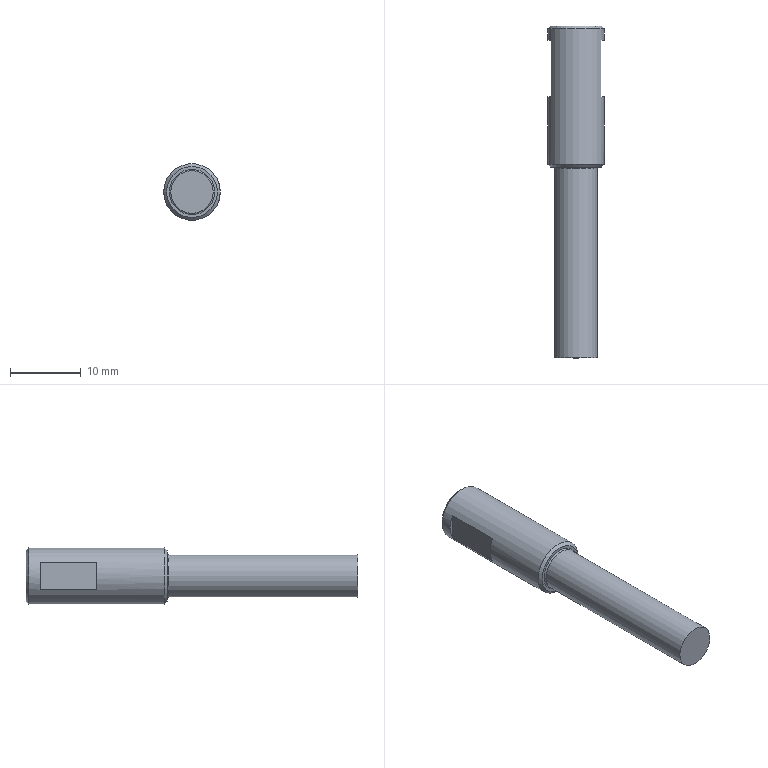Part | NX | features 5003_002_SFRNS8-20.0-F27.0-B13-P6-SC10 2 | 1 solid | 14 faces | box 8 x 47 x 8 mm | volume 1744 mm3 | plane 9 | cylinder 2 | cone 2 | torus 1 | commonest cylinder face diameters 6 x1 8 x1
STEP:
#1=CARTESIAN_POINT('',(-212.775,-579.,-110.5));
#2=VERTEX_POINT('',#1);
#3=CARTESIAN_POINT('',(-216.775,-579.,-110.5));
#4=DIRECTION('',(0.,-1.,0.));
#5=DIRECTION('',(1.,0.,0.));
#6=AXIS2_PLACEMENT_3D('',#3,#4,#5);
#7=CIRCLE('',#6,4.);
#8=EDGE_CURVE('',#2,#2,#7,.T.);
#9=ORIENTED_EDGE('',*,*,#8,.T.);
#10=EDGE_LOOP('',(#9));
#11=FACE_BOUND('',#10,.T.);
#12=CARTESIAN_POINT('',(-220.775,-598.2,-110.5));
#13=VERTEX_POINT('',#12);
#14=CARTESIAN_POINT('',(-216.775,-598.2,-110.5));
#15=DIRECTION('',(0.,1.,0.));
#16=DIRECTION('',(-1.,0.,0.));
#17=AXIS2_PLACEMENT_3D('',#14,#15,#16);
#18=CIRCLE('',#17,4.);
#19=EDGE_CURVE('',#13,#13,#18,.T.);
#20=ORIENTED_EDGE('',*,*,#19,.T.);
#21=EDGE_LOOP('',(#20));
#22=FACE_BOUND('',#21,.T.);
#23=CARTESIAN_POINT('',(-213.275,-580.6,-108.564));
#24=VERTEX_POINT('',#23);
#25=CARTESIAN_POINT('',(-213.275,-588.6,-108.564));
#26=VERTEX_POINT('',#25);
#27=CARTESIAN_POINT('',(-213.275,-625.6,-108.564));
#28=DIRECTION('',(0.,-1.,0.));
#29=VECTOR('',#28,1000.);
#30=LINE('',#27,#29);
#31=EDGE_CURVE('',#24,#26,#30,.T.);
#32=ORIENTED_EDGE('',*,*,#31,.F.);
#33=CARTESIAN_POINT('',(-213.275,-580.6,-112.436));
#34=VERTEX_POINT('',#33);
#35=CARTESIAN_POINT('',(-216.775,-580.6,-110.5));
#36=DIRECTION('',(0.,-1.,0.));
#37=DIRECTION('',(1.,0.,0.));
#38=AXIS2_PLACEMENT_3D('',#35,#36,#37);
#39=CIRCLE('',#38,4.);
#40=EDGE_CURVE('',#34,#24,#39,.T.);
#41=ORIENTED_EDGE('',*,*,#40,.F.);
#42=CARTESIAN_POINT('',(-213.275,-588.6,-112.436));
#43=VERTEX_POINT('',#42);
#44=CARTESIAN_POINT('',(-213.275,-625.6,-112.436));
#45=DIRECTION('',(0.,-1.,0.));
#46=VECTOR('',#45,1000.);
#47=LINE('',#44,#46);
#48=EDGE_CURVE('',#43,#34,#47,.F.);
#49=ORIENTED_EDGE('',*,*,#48,.F.);
#50=CARTESIAN_POINT('',(-216.775,-588.6,-110.5));
#51=DIRECTION('',(0.,1.,0.));
#52=DIRECTION('',(-1.,0.,0.));
#53=AXIS2_PLACEMENT_3D('',#50,#51,#52);
#54=CIRCLE('',#53,4.);
#55=EDGE_CURVE('',#26,#43,#54,.T.);
#56=ORIENTED_EDGE('',*,*,#55,.F.);
#57=EDGE_LOOP('',(#32,#41,#49,#56));
#58=FACE_BOUND('',#57,.T.);
#59=CARTESIAN_POINT('',(-220.275,-580.6,-108.564));
#60=VERTEX_POINT('',#59);
#61=CARTESIAN_POINT('',(-220.275,-580.6,-112.436));
#62=VERTEX_POINT('',#61);
#63=CARTESIAN_POINT('',(-216.775,-580.6,-110.5));
#64=DIRECTION('',(0.,-1.,0.));
#65=DIRECTION('',(1.,0.,0.));
#66=AXIS2_PLACEMENT_3D('',#63,#64,#65);
#67=CIRCLE('',#66,4.);
#68=EDGE_CURVE('',#60,#62,#67,.T.);
#69=ORIENTED_EDGE('',*,*,#68,.F.);
#70=CARTESIAN_POINT('',(-220.275,-588.6,-108.564));
#71=VERTEX_POINT('',#70);
#72=CARTESIAN_POINT('',(-220.275,-625.6,-108.564));
#73=DIRECTION('',(0.,-1.,0.));
#74=VECTOR('',#73,1000.);
#75=LINE('',#72,#74);
#76=EDGE_CURVE('',#71,#60,#75,.F.);
#77=ORIENTED_EDGE('',*,*,#76,.F.);
#78=CARTESIAN_POINT('',(-220.275,-588.6,-112.436));
#79=VERTEX_POINT('',#78);
#80=CARTESIAN_POINT('',(-216.775,-588.6,-110.5));
#81=DIRECTION('',(0.,1.,0.));
#82=DIRECTION('',(-1.,0.,0.));
#83=AXIS2_PLACEMENT_3D('',#80,#81,#82);
#84=CIRCLE('',#83,4.);
#85=EDGE_CURVE('',#79,#71,#84,.T.);
#86=ORIENTED_EDGE('',*,*,#85,.F.);
#87=CARTESIAN_POINT('',(-220.275,-625.6,-112.436));
#88=DIRECTION('',(0.,-1.,0.));
#89=VECTOR('',#88,1000.);
#90=LINE('',#87,#89);
#91=EDGE_CURVE('',#62,#79,#90,.T.);
#92=ORIENTED_EDGE('',*,*,#91,.F.);
#93=EDGE_LOOP('',(#69,#77,#86,#92));
#94=FACE_BOUND('',#93,.T.);
#95=CARTESIAN_POINT('',(-216.775,-625.6,-110.5));
#96=DIRECTION('',(0.,-1.,0.));
#97=DIRECTION('',(1.,0.,0.));
#98=AXIS2_PLACEMENT_3D('',#95,#96,#97);
#99=CYLINDRICAL_SURFACE('',#98,4.);
#100=ADVANCED_FACE('',(#11,#22,#58,#94),#99,.T.);
#101=CARTESIAN_POINT('',(-213.175,-578.6,-110.5));
#102=VERTEX_POINT('',#101);
#103=CARTESIAN_POINT('',(-216.775,-578.6,-110.5));
#104=DIRECTION('',(0.,-1.,0.));
#105=DIRECTION('',(1.,0.,0.));
#106=AXIS2_PLACEMENT_3D('',#103,#104,#105);
#107=CIRCLE('',#106,3.6);
#108=EDGE_CURVE('',#102,#102,#107,.F.);
#109=ORIENTED_EDGE('',*,*,#108,.T.);
#110=EDGE_LOOP('',(#109));
#111=FACE_BOUND('',#110,.T.);
#112=CARTESIAN_POINT('',(-216.775,-578.6,-110.5));
#113=DIRECTION('',(0.,-1.,0.));
#114=DIRECTION('',(1.,0.,0.));
#115=AXIS2_PLACEMENT_3D('',#112,#113,#114);
#116=PLANE('',#115);
#117=ADVANCED_FACE('',(#111),#116,.F.);
#118=CARTESIAN_POINT('',(-219.975,-598.6,-110.5));
#119=VERTEX_POINT('',#118);
#120=CARTESIAN_POINT('',(-216.775,-598.6,-110.5));
#121=DIRECTION('',(0.,1.,0.));
#122=DIRECTION('',(-1.,0.,0.));
#123=AXIS2_PLACEMENT_3D('',#120,#121,#122);
#124=CIRCLE('',#123,3.2);
#125=EDGE_CURVE('',#119,#119,#124,.T.);
#126=ORIENTED_EDGE('',*,*,#125,.T.);
#127=EDGE_LOOP('',(#126));
#128=FACE_BOUND('',#127,.T.);
#129=CARTESIAN_POINT('',(-220.375,-598.6,-110.5));
#130=VERTEX_POINT('',#129);
#131=CARTESIAN_POINT('',(-216.775,-598.6,-110.5));
#132=DIRECTION('',(0.,1.,0.));
#133=DIRECTION('',(-1.,0.,0.));
#134=AXIS2_PLACEMENT_3D('',#131,#132,#133);
#135=CIRCLE('',#134,3.6);
#136=EDGE_CURVE('',#130,#130,#135,.F.);
#137=ORIENTED_EDGE('',*,*,#136,.T.);
#138=EDGE_LOOP('',(#137));
#139=FACE_BOUND('',#138,.T.);
#140=CARTESIAN_POINT('',(-216.775,-598.6,-106.5));
#141=DIRECTION('',(0.,1.,0.));
#142=DIRECTION('',(-1.,0.,0.));
#143=AXIS2_PLACEMENT_3D('',#140,#141,#142);
#144=PLANE('',#143);
#145=ADVANCED_FACE('',(#128,#139),#144,.F.);
#146=CARTESIAN_POINT('',(-219.775,-598.8,-110.5));
#147=VERTEX_POINT('',#146);
#148=CARTESIAN_POINT('',(-216.775,-598.8,-110.5));
#149=DIRECTION('',(0.,1.,0.));
#150=DIRECTION('',(-1.,0.,0.));
#151=AXIS2_PLACEMENT_3D('',#148,#149,#150);
#152=CIRCLE('',#151,3.);
#153=EDGE_CURVE('',#147,#147,#152,.F.);
#154=ORIENTED_EDGE('',*,*,#153,.T.);
#155=EDGE_LOOP('',(#154));
#156=FACE_BOUND('',#155,.T.);
#157=CARTESIAN_POINT('',(-213.775,-625.6,-110.5));
#158=VERTEX_POINT('',#157);
#159=CARTESIAN_POINT('',(-216.775,-625.6,-110.5));
#160=DIRECTION('',(0.,-1.,0.));
#161=DIRECTION('',(1.,0.,0.));
#162=AXIS2_PLACEMENT_3D('',#159,#160,#161);
#163=CIRCLE('',#162,3.);
#164=EDGE_CURVE('',#158,#158,#163,.T.);
#165=ORIENTED_EDGE('',*,*,#164,.F.);
#166=EDGE_LOOP('',(#165));
#167=FACE_BOUND('',#166,.T.);
#168=CARTESIAN_POINT('',(-216.775,-625.6,-110.5));
#169=DIRECTION('',(0.,-1.,0.));
#170=DIRECTION('',(1.,0.,0.));
#171=AXIS2_PLACEMENT_3D('',#168,#169,#170);
#172=CYLINDRICAL_SURFACE('',#171,3.);
#173=ADVANCED_FACE('',(#156,#167),#172,.T.);
#174=ORIENTED_EDGE('',*,*,#164,.T.);
#175=EDGE_LOOP('',(#174));
#176=FACE_BOUND('',#175,.T.);
#177=CARTESIAN_POINT('',(-216.775,-625.6,-107.5));
#178=DIRECTION('',(0.,1.,0.));
#179=DIRECTION('',(-1.,0.,0.));
#180=AXIS2_PLACEMENT_3D('',#177,#178,#179);
#181=PLANE('',#180);
#182=ADVANCED_FACE('',(#176),#181,.F.);
#183=ORIENTED_EDGE('',*,*,#108,.F.);
#184=EDGE_LOOP('',(#183));
#185=FACE_BOUND('',#184,.T.);
#186=ORIENTED_EDGE('',*,*,#8,.F.);
#187=EDGE_LOOP('',(#186));
#188=FACE_BOUND('',#187,.T.);
#189=CARTESIAN_POINT('',(-216.775,-579.,-110.5));
#190=DIRECTION('',(0.,-1.,0.));
#191=DIRECTION('',(1.,0.,0.));
#192=AXIS2_PLACEMENT_3D('',#189,#190,#191);
#193=CONICAL_SURFACE('',#192,4.,0.7854);
#194=ADVANCED_FACE('',(#185,#188),#193,.T.);
#195=ORIENTED_EDGE('',*,*,#19,.F.);
#196=EDGE_LOOP('',(#195));
#197=FACE_BOUND('',#196,.T.);
#198=ORIENTED_EDGE('',*,*,#136,.F.);
#199=EDGE_LOOP('',(#198));
#200=FACE_BOUND('',#199,.T.);
#201=CARTESIAN_POINT('',(-216.775,-598.6,-110.5));
#202=DIRECTION('',(0.,1.,0.));
#203=DIRECTION('',(-1.,0.,0.));
#204=AXIS2_PLACEMENT_3D('',#201,#202,#203);
#205=CONICAL_SURFACE('',#204,3.6,0.7854);
#206=ADVANCED_FACE('',(#197,#200),#205,.T.);
#207=ORIENTED_EDGE('',*,*,#125,.F.);
#208=EDGE_LOOP('',(#207));
#209=FACE_BOUND('',#208,.T.);
#210=ORIENTED_EDGE('',*,*,#153,.F.);
#211=EDGE_LOOP('',(#210));
#212=FACE_BOUND('',#211,.T.);
#213=CARTESIAN_POINT('',(-216.775,-598.8,-110.5));
#214=DIRECTION('',(0.,1.,0.));
#215=DIRECTION('',(-1.,0.,0.));
#216=AXIS2_PLACEMENT_3D('',#213,#214,#215);
#217=TOROIDAL_SURFACE('',#216,3.2,0.2);
#218=ADVANCED_FACE('',(#209,#212),#217,.F.);
#219=CARTESIAN_POINT('',(-213.275,-588.6,-106.5));
#220=DIRECTION('',(0.,0.,-1.));
#221=VECTOR('',#220,1000.);
#222=LINE('',#219,#221);
#223=EDGE_CURVE('',#26,#43,#222,.T.);
#224=ORIENTED_EDGE('',*,*,#223,.F.);
#225=ORIENTED_EDGE('',*,*,#55,.T.);
#226=EDGE_LOOP('',(#224,#225));
#227=FACE_BOUND('',#226,.T.);
#228=CARTESIAN_POINT('',(-213.275,-588.6,-106.5));
#229=DIRECTION('',(0.,1.,0.));
#230=DIRECTION('',(-1.,0.,0.));
#231=AXIS2_PLACEMENT_3D('',#228,#229,#230);
#232=PLANE('',#231);
#233=ADVANCED_FACE('',(#227),#232,.T.);
#234=ORIENTED_EDGE('',*,*,#40,.T.);
#235=CARTESIAN_POINT('',(-213.275,-580.6,-106.5));
#236=DIRECTION('',(0.,0.,-1.));
#237=VECTOR('',#236,1000.);
#238=LINE('',#235,#237);
#239=EDGE_CURVE('',#24,#34,#238,.T.);
#240=ORIENTED_EDGE('',*,*,#239,.T.);
#241=EDGE_LOOP('',(#234,#240));
#242=FACE_BOUND('',#241,.T.);
#243=CARTESIAN_POINT('',(-213.275,-580.6,-106.5));
#244=DIRECTION('',(0.,-1.,0.));
#245=DIRECTION('',(1.,0.,0.));
#246=AXIS2_PLACEMENT_3D('',#243,#244,#245);
#247=PLANE('',#246);
#248=ADVANCED_FACE('',(#242),#247,.T.);
#249=ORIENTED_EDGE('',*,*,#31,.T.);
#250=ORIENTED_EDGE('',*,*,#223,.T.);
#251=ORIENTED_EDGE('',*,*,#48,.T.);
#252=ORIENTED_EDGE('',*,*,#239,.F.);
#253=EDGE_LOOP('',(#249,#250,#251,#252));
#254=FACE_BOUND('',#253,.T.);
#255=CARTESIAN_POINT('',(-213.275,-588.6,-106.5));
#256=DIRECTION('',(1.,0.,0.));
#257=DIRECTION('',(0.,1.,0.));
#258=AXIS2_PLACEMENT_3D('',#255,#256,#257);
#259=PLANE('',#258);
#260=ADVANCED_FACE('',(#254),#259,.T.);
#261=ORIENTED_EDGE('',*,*,#85,.T.);
#262=CARTESIAN_POINT('',(-220.275,-588.6,-106.5));
#263=DIRECTION('',(0.,0.,-1.));
#264=VECTOR('',#263,1000.);
#265=LINE('',#262,#264);
#266=EDGE_CURVE('',#71,#79,#265,.T.);
#267=ORIENTED_EDGE('',*,*,#266,.T.);
#268=EDGE_LOOP('',(#261,#267));
#269=FACE_BOUND('',#268,.T.);
#270=CARTESIAN_POINT('',(-220.775,-588.6,-106.5));
#271=DIRECTION('',(0.,1.,0.));
#272=DIRECTION('',(-1.,0.,0.));
#273=AXIS2_PLACEMENT_3D('',#270,#271,#272);
#274=PLANE('',#273);
#275=ADVANCED_FACE('',(#269),#274,.T.);
#276=ORIENTED_EDGE('',*,*,#91,.T.);
#277=ORIENTED_EDGE('',*,*,#266,.F.);
#278=ORIENTED_EDGE('',*,*,#76,.T.);
#279=CARTESIAN_POINT('',(-220.275,-580.6,-106.5));
#280=DIRECTION('',(0.,0.,-1.));
#281=VECTOR('',#280,1000.);
#282=LINE('',#279,#281);
#283=EDGE_CURVE('',#60,#62,#282,.T.);
#284=ORIENTED_EDGE('',*,*,#283,.T.);
#285=EDGE_LOOP('',(#276,#277,#278,#284));
#286=FACE_BOUND('',#285,.T.);
#287=CARTESIAN_POINT('',(-220.275,-588.6,-106.5));
#288=DIRECTION('',(-1.,0.,0.));
#289=DIRECTION('',(0.,-1.,0.));
#290=AXIS2_PLACEMENT_3D('',#287,#288,#289);
#291=PLANE('',#290);
#292=ADVANCED_FACE('',(#286),#291,.T.);
#293=ORIENTED_EDGE('',*,*,#283,.F.);
#294=ORIENTED_EDGE('',*,*,#68,.T.);
#295=EDGE_LOOP('',(#293,#294));
#296=FACE_BOUND('',#295,.T.);
#297=CARTESIAN_POINT('',(-220.775,-580.6,-106.5));
#298=DIRECTION('',(0.,-1.,0.));
#299=DIRECTION('',(1.,0.,0.));
#300=AXIS2_PLACEMENT_3D('',#297,#298,#299);
#301=PLANE('',#300);
#302=ADVANCED_FACE('',(#296),#301,.T.);
#303=CLOSED_SHELL('',(#100,#117,#145,#173,#182,#194,#206,#218,#233,#248,#260,#275,#292,#302));
#304=MANIFOLD_SOLID_BREP('',#303);
#305=(LENGTH_UNIT()NAMED_UNIT(*)SI_UNIT(.MILLI.,.METRE.));
#306=UNCERTAINTY_MEASURE_WITH_UNIT(LENGTH_MEASURE(0.00001),#305,'','');
#307=(NAMED_UNIT(*)PLANE_ANGLE_UNIT()SI_UNIT($,.RADIAN.));
#308=(NAMED_UNIT(*)SI_UNIT($,.STERADIAN.)SOLID_ANGLE_UNIT());
#309=(GEOMETRIC_REPRESENTATION_CONTEXT(3)GLOBAL_UNCERTAINTY_ASSIGNED_CONTEXT((#306))GLOBAL_UNIT_ASSIGNED_CONTEXT((#305,#307,#308))REPRESENTATION_CONTEXT('',''));
#310=ADVANCED_BREP_SHAPE_REPRESENTATION('',(#304),#309);